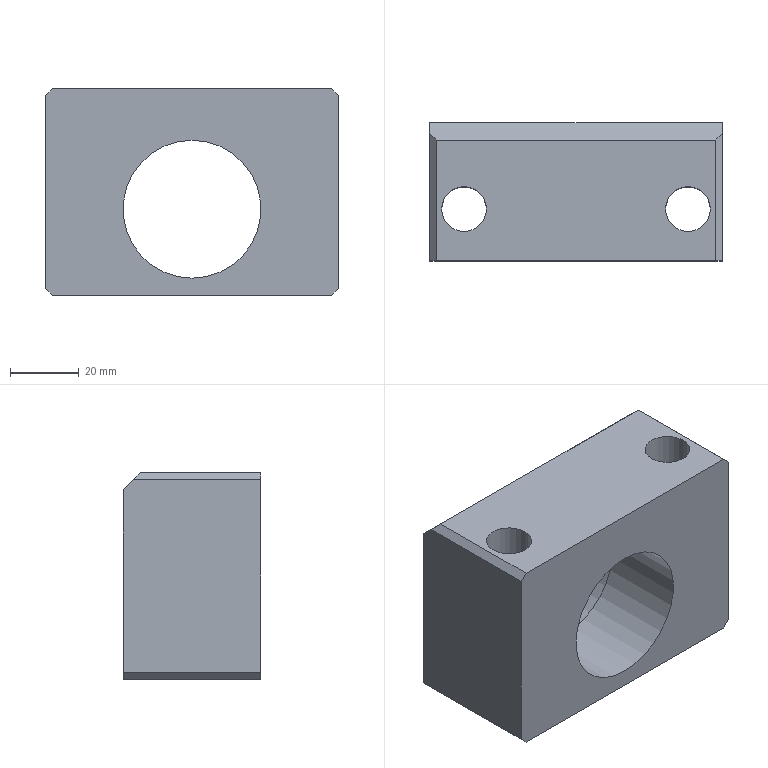Part | NX | features solid 2 | 1 solid | 16 faces | box 85 x 40 x 60 mm | volume 131435 mm3 | plane 12 | cylinder 4 | commonest cylinder face diameters 13 x2 40 x1 45 x1
STEP:
#1=CARTESIAN_POINT('',(521.,750.,75.));
#2=VERTEX_POINT('',#1);
#3=CARTESIAN_POINT('',(527.5,750.,75.));
#4=DIRECTION('',(0.,0.,-1.));
#5=DIRECTION('',(-1.,0.,0.));
#6=AXIS2_PLACEMENT_3D('',#3,#4,#5);
#7=CIRCLE('',#6,6.5);
#8=EDGE_CURVE('',#2,#2,#7,.T.);
#9=ORIENTED_EDGE('',*,*,#8,.F.);
#10=EDGE_LOOP('',(#9));
#11=FACE_BOUND('',#10,.T.);
#12=CARTESIAN_POINT('',(456.,750.,75.));
#13=VERTEX_POINT('',#12);
#14=CARTESIAN_POINT('',(462.5,750.,75.));
#15=DIRECTION('',(0.,0.,-1.));
#16=DIRECTION('',(-1.,0.,0.));
#17=AXIS2_PLACEMENT_3D('',#14,#15,#16);
#18=CIRCLE('',#17,6.5);
#19=EDGE_CURVE('',#13,#13,#18,.T.);
#20=ORIENTED_EDGE('',*,*,#19,.F.);
#21=EDGE_LOOP('',(#20));
#22=FACE_BOUND('',#21,.T.);
#23=CARTESIAN_POINT('',(535.5,735.,75.));
#24=VERTEX_POINT('',#23);
#25=CARTESIAN_POINT('',(454.5,735.,75.));
#26=VERTEX_POINT('',#25);
#27=CARTESIAN_POINT('',(495.,735.,75.));
#28=DIRECTION('',(-1.,0.,0.));
#29=VECTOR('',#28,1000.);
#30=LINE('',#27,#29);
#31=EDGE_CURVE('',#24,#26,#30,.T.);
#32=ORIENTED_EDGE('',*,*,#31,.T.);
#33=CARTESIAN_POINT('',(454.5,775.,75.));
#34=VERTEX_POINT('',#33);
#35=CARTESIAN_POINT('',(454.5,755.,75.));
#36=DIRECTION('',(0.,-1.,0.));
#37=VECTOR('',#36,1000.);
#38=LINE('',#35,#37);
#39=EDGE_CURVE('',#34,#26,#38,.T.);
#40=ORIENTED_EDGE('',*,*,#39,.F.);
#41=CARTESIAN_POINT('',(535.5,775.,75.));
#42=VERTEX_POINT('',#41);
#43=CARTESIAN_POINT('',(495.,775.,75.));
#44=DIRECTION('',(1.,0.,0.));
#45=VECTOR('',#44,1000.);
#46=LINE('',#43,#45);
#47=EDGE_CURVE('',#34,#42,#46,.T.);
#48=ORIENTED_EDGE('',*,*,#47,.T.);
#49=CARTESIAN_POINT('',(535.5,755.,75.));
#50=DIRECTION('',(0.,1.,0.));
#51=VECTOR('',#50,1000.);
#52=LINE('',#49,#51);
#53=EDGE_CURVE('',#24,#42,#52,.T.);
#54=ORIENTED_EDGE('',*,*,#53,.F.);
#55=EDGE_LOOP('',(#32,#40,#48,#54));
#56=FACE_BOUND('',#55,.T.);
#57=CARTESIAN_POINT('',(495.,755.,75.));
#58=DIRECTION('',(0.,0.,-1.));
#59=DIRECTION('',(1.,0.,0.));
#60=AXIS2_PLACEMENT_3D('',#57,#58,#59);
#61=PLANE('',#60);
#62=ADVANCED_FACE('',(#11,#22,#56),#61,.T.);
#63=CARTESIAN_POINT('',(495.,735.,120.));
#64=VERTEX_POINT('',#63);
#65=CARTESIAN_POINT('',(495.,735.,100.));
#66=DIRECTION('',(0.,1.,0.));
#67=DIRECTION('',(0.,0.,1.));
#68=AXIS2_PLACEMENT_3D('',#65,#66,#67);
#69=CIRCLE('',#68,20.);
#70=EDGE_CURVE('',#64,#64,#69,.T.);
#71=ORIENTED_EDGE('',*,*,#70,.T.);
#72=EDGE_LOOP('',(#71));
#73=FACE_BOUND('',#72,.T.);
#74=CARTESIAN_POINT('',(452.5,735.,133.));
#75=VERTEX_POINT('',#74);
#76=CARTESIAN_POINT('',(452.5,735.,77.));
#77=VERTEX_POINT('',#76);
#78=CARTESIAN_POINT('',(452.5,735.,135.));
#79=DIRECTION('',(0.,0.,-1.));
#80=VECTOR('',#79,1000.);
#81=LINE('',#78,#80);
#82=EDGE_CURVE('',#75,#77,#81,.T.);
#83=ORIENTED_EDGE('',*,*,#82,.T.);
#84=CARTESIAN_POINT('',(444.75,735.,84.75));
#85=DIRECTION('',(0.7071,0.,-0.7071));
#86=VECTOR('',#85,1000.);
#87=LINE('',#84,#86);
#88=EDGE_CURVE('',#26,#77,#87,.F.);
#89=ORIENTED_EDGE('',*,*,#88,.F.);
#90=ORIENTED_EDGE('',*,*,#31,.F.);
#91=CARTESIAN_POINT('',(537.5,735.,77.));
#92=VERTEX_POINT('',#91);
#93=CARTESIAN_POINT('',(545.25,735.,84.75));
#94=DIRECTION('',(0.7071,0.,0.7071));
#95=VECTOR('',#94,1000.);
#96=LINE('',#93,#95);
#97=EDGE_CURVE('',#92,#24,#96,.F.);
#98=ORIENTED_EDGE('',*,*,#97,.F.);
#99=CARTESIAN_POINT('',(537.5,735.,133.));
#100=VERTEX_POINT('',#99);
#101=CARTESIAN_POINT('',(537.5,735.,135.));
#102=DIRECTION('',(0.,0.,-1.));
#103=VECTOR('',#102,1000.);
#104=LINE('',#101,#103);
#105=EDGE_CURVE('',#100,#92,#104,.T.);
#106=ORIENTED_EDGE('',*,*,#105,.F.);
#107=CARTESIAN_POINT('',(535.5,735.,135.));
#108=VERTEX_POINT('',#107);
#109=CARTESIAN_POINT('',(515.25,735.,155.25));
#110=DIRECTION('',(-0.7071,0.,0.7071));
#111=VECTOR('',#110,1000.);
#112=LINE('',#109,#111);
#113=EDGE_CURVE('',#108,#100,#112,.F.);
#114=ORIENTED_EDGE('',*,*,#113,.F.);
#115=CARTESIAN_POINT('',(454.5,735.,135.));
#116=VERTEX_POINT('',#115);
#117=CARTESIAN_POINT('',(495.,735.,135.));
#118=DIRECTION('',(1.,0.,0.));
#119=VECTOR('',#118,1000.);
#120=LINE('',#117,#119);
#121=EDGE_CURVE('',#116,#108,#120,.T.);
#122=ORIENTED_EDGE('',*,*,#121,.F.);
#123=CARTESIAN_POINT('',(474.75,735.,155.25));
#124=DIRECTION('',(-0.7071,0.,-0.7071));
#125=VECTOR('',#124,1000.);
#126=LINE('',#123,#125);
#127=EDGE_CURVE('',#75,#116,#126,.F.);
#128=ORIENTED_EDGE('',*,*,#127,.F.);
#129=EDGE_LOOP('',(#83,#89,#90,#98,#106,#114,#122,#128));
#130=FACE_BOUND('',#129,.T.);
#131=CARTESIAN_POINT('',(495.,735.,135.));
#132=DIRECTION('',(0.,-1.,0.));
#133=DIRECTION('',(0.,0.,1.));
#134=AXIS2_PLACEMENT_3D('',#131,#132,#133);
#135=PLANE('',#134);
#136=ADVANCED_FACE('',(#73,#130),#135,.T.);
#137=CARTESIAN_POINT('',(452.5,775.,130.));
#138=VERTEX_POINT('',#137);
#139=CARTESIAN_POINT('',(452.5,772.,133.));
#140=VERTEX_POINT('',#139);
#141=CARTESIAN_POINT('',(452.5,762.5,142.5));
#142=DIRECTION('',(0.,0.7071,-0.7071));
#143=VECTOR('',#142,1000.);
#144=LINE('',#141,#143);
#145=EDGE_CURVE('',#138,#140,#144,.F.);
#146=ORIENTED_EDGE('',*,*,#145,.F.);
#147=CARTESIAN_POINT('',(452.5,775.,77.));
#148=VERTEX_POINT('',#147);
#149=CARTESIAN_POINT('',(452.5,775.,135.));
#150=DIRECTION('',(0.,0.,-1.));
#151=VECTOR('',#150,1000.);
#152=LINE('',#149,#151);
#153=EDGE_CURVE('',#138,#148,#152,.T.);
#154=ORIENTED_EDGE('',*,*,#153,.T.);
#155=CARTESIAN_POINT('',(452.5,755.,77.));
#156=DIRECTION('',(0.,1.,0.));
#157=VECTOR('',#156,1000.);
#158=LINE('',#155,#157);
#159=EDGE_CURVE('',#77,#148,#158,.T.);
#160=ORIENTED_EDGE('',*,*,#159,.F.);
#161=ORIENTED_EDGE('',*,*,#82,.F.);
#162=CARTESIAN_POINT('',(452.5,755.,133.));
#163=DIRECTION('',(0.,-1.,0.));
#164=VECTOR('',#163,1000.);
#165=LINE('',#162,#164);
#166=EDGE_CURVE('',#140,#75,#165,.T.);
#167=ORIENTED_EDGE('',*,*,#166,.F.);
#168=EDGE_LOOP('',(#146,#154,#160,#161,#167));
#169=FACE_BOUND('',#168,.T.);
#170=CARTESIAN_POINT('',(452.5,755.,135.));
#171=DIRECTION('',(-1.,0.,0.));
#172=DIRECTION('',(0.,0.,-1.));
#173=AXIS2_PLACEMENT_3D('',#170,#171,#172);
#174=PLANE('',#173);
#175=ADVANCED_FACE('',(#169),#174,.T.);
#176=CARTESIAN_POINT('',(495.,775.,122.5));
#177=VERTEX_POINT('',#176);
#178=CARTESIAN_POINT('',(495.,775.,100.));
#179=DIRECTION('',(0.,1.,0.));
#180=DIRECTION('',(0.,0.,1.));
#181=AXIS2_PLACEMENT_3D('',#178,#179,#180);
#182=CIRCLE('',#181,22.5);
#183=EDGE_CURVE('',#177,#177,#182,.T.);
#184=ORIENTED_EDGE('',*,*,#183,.F.);
#185=EDGE_LOOP('',(#184));
#186=FACE_BOUND('',#185,.T.);
#187=ORIENTED_EDGE('',*,*,#47,.F.);
#188=CARTESIAN_POINT('',(444.75,775.,84.75));
#189=DIRECTION('',(-0.7071,0.,0.7071));
#190=VECTOR('',#189,1000.);
#191=LINE('',#188,#190);
#192=EDGE_CURVE('',#148,#34,#191,.F.);
#193=ORIENTED_EDGE('',*,*,#192,.F.);
#194=ORIENTED_EDGE('',*,*,#153,.F.);
#195=CARTESIAN_POINT('',(537.5,775.,130.));
#196=VERTEX_POINT('',#195);
#197=CARTESIAN_POINT('',(495.,775.,130.));
#198=DIRECTION('',(-1.,0.,0.));
#199=VECTOR('',#198,1000.);
#200=LINE('',#197,#199);
#201=EDGE_CURVE('',#196,#138,#200,.T.);
#202=ORIENTED_EDGE('',*,*,#201,.F.);
#203=CARTESIAN_POINT('',(537.5,775.,77.));
#204=VERTEX_POINT('',#203);
#205=CARTESIAN_POINT('',(537.5,775.,135.));
#206=DIRECTION('',(0.,0.,-1.));
#207=VECTOR('',#206,1000.);
#208=LINE('',#205,#207);
#209=EDGE_CURVE('',#196,#204,#208,.T.);
#210=ORIENTED_EDGE('',*,*,#209,.T.);
#211=CARTESIAN_POINT('',(545.25,775.,84.75));
#212=DIRECTION('',(-0.7071,0.,-0.7071));
#213=VECTOR('',#212,1000.);
#214=LINE('',#211,#213);
#215=EDGE_CURVE('',#42,#204,#214,.F.);
#216=ORIENTED_EDGE('',*,*,#215,.F.);
#217=EDGE_LOOP('',(#187,#193,#194,#202,#210,#216));
#218=FACE_BOUND('',#217,.T.);
#219=CARTESIAN_POINT('',(495.,775.,135.));
#220=DIRECTION('',(0.,1.,0.));
#221=DIRECTION('',(0.,0.,-1.));
#222=AXIS2_PLACEMENT_3D('',#219,#220,#221);
#223=PLANE('',#222);
#224=ADVANCED_FACE('',(#186,#218),#223,.T.);
#225=CARTESIAN_POINT('',(521.,750.,135.));
#226=VERTEX_POINT('',#225);
#227=CARTESIAN_POINT('',(527.5,750.,135.));
#228=DIRECTION('',(0.,0.,-1.));
#229=DIRECTION('',(-1.,0.,0.));
#230=AXIS2_PLACEMENT_3D('',#227,#228,#229);
#231=CIRCLE('',#230,6.5);
#232=EDGE_CURVE('',#226,#226,#231,.T.);
#233=ORIENTED_EDGE('',*,*,#232,.T.);
#234=EDGE_LOOP('',(#233));
#235=FACE_BOUND('',#234,.T.);
#236=CARTESIAN_POINT('',(456.,750.,135.));
#237=VERTEX_POINT('',#236);
#238=CARTESIAN_POINT('',(462.5,750.,135.));
#239=DIRECTION('',(0.,0.,-1.));
#240=DIRECTION('',(-1.,0.,0.));
#241=AXIS2_PLACEMENT_3D('',#238,#239,#240);
#242=CIRCLE('',#241,6.5);
#243=EDGE_CURVE('',#237,#237,#242,.T.);
#244=ORIENTED_EDGE('',*,*,#243,.T.);
#245=EDGE_LOOP('',(#244));
#246=FACE_BOUND('',#245,.T.);
#247=ORIENTED_EDGE('',*,*,#121,.T.);
#248=CARTESIAN_POINT('',(535.5,770.,135.));
#249=VERTEX_POINT('',#248);
#250=CARTESIAN_POINT('',(535.5,755.,135.));
#251=DIRECTION('',(0.,-1.,0.));
#252=VECTOR('',#251,1000.);
#253=LINE('',#250,#252);
#254=EDGE_CURVE('',#249,#108,#253,.T.);
#255=ORIENTED_EDGE('',*,*,#254,.F.);
#256=CARTESIAN_POINT('',(454.5,770.,135.));
#257=VERTEX_POINT('',#256);
#258=CARTESIAN_POINT('',(495.,770.,135.));
#259=DIRECTION('',(1.,0.,0.));
#260=VECTOR('',#259,1000.);
#261=LINE('',#258,#260);
#262=EDGE_CURVE('',#257,#249,#261,.T.);
#263=ORIENTED_EDGE('',*,*,#262,.F.);
#264=CARTESIAN_POINT('',(454.5,755.,135.));
#265=DIRECTION('',(0.,1.,0.));
#266=VECTOR('',#265,1000.);
#267=LINE('',#264,#266);
#268=EDGE_CURVE('',#116,#257,#267,.T.);
#269=ORIENTED_EDGE('',*,*,#268,.F.);
#270=EDGE_LOOP('',(#247,#255,#263,#269));
#271=FACE_BOUND('',#270,.T.);
#272=CARTESIAN_POINT('',(495.,755.,135.));
#273=DIRECTION('',(0.,0.,1.));
#274=DIRECTION('',(-1.,0.,0.));
#275=AXIS2_PLACEMENT_3D('',#272,#273,#274);
#276=PLANE('',#275);
#277=ADVANCED_FACE('',(#235,#246,#271),#276,.T.);
#278=ORIENTED_EDGE('',*,*,#105,.T.);
#279=CARTESIAN_POINT('',(537.5,755.,77.));
#280=DIRECTION('',(0.,-1.,0.));
#281=VECTOR('',#280,1000.);
#282=LINE('',#279,#281);
#283=EDGE_CURVE('',#204,#92,#282,.T.);
#284=ORIENTED_EDGE('',*,*,#283,.F.);
#285=ORIENTED_EDGE('',*,*,#209,.F.);
#286=CARTESIAN_POINT('',(537.5,772.,133.));
#287=VERTEX_POINT('',#286);
#288=CARTESIAN_POINT('',(537.5,762.5,142.5));
#289=DIRECTION('',(0.,-0.7071,0.7071));
#290=VECTOR('',#289,1000.);
#291=LINE('',#288,#290);
#292=EDGE_CURVE('',#287,#196,#291,.F.);
#293=ORIENTED_EDGE('',*,*,#292,.F.);
#294=CARTESIAN_POINT('',(537.5,755.,133.));
#295=DIRECTION('',(0.,1.,0.));
#296=VECTOR('',#295,1000.);
#297=LINE('',#294,#296);
#298=EDGE_CURVE('',#100,#287,#297,.T.);
#299=ORIENTED_EDGE('',*,*,#298,.F.);
#300=EDGE_LOOP('',(#278,#284,#285,#293,#299));
#301=FACE_BOUND('',#300,.T.);
#302=CARTESIAN_POINT('',(537.5,755.,135.));
#303=DIRECTION('',(1.,0.,0.));
#304=DIRECTION('',(0.,0.,1.));
#305=AXIS2_PLACEMENT_3D('',#302,#303,#304);
#306=PLANE('',#305);
#307=ADVANCED_FACE('',(#301),#306,.T.);
#308=ORIENTED_EDGE('',*,*,#262,.T.);
#309=CARTESIAN_POINT('',(525.333,759.833,145.167));
#310=DIRECTION('',(-0.5774,-0.5774,0.5774));
#311=VECTOR('',#310,1000.);
#312=LINE('',#309,#311);
#313=EDGE_CURVE('',#287,#249,#312,.T.);
#314=ORIENTED_EDGE('',*,*,#313,.F.);
#315=ORIENTED_EDGE('',*,*,#292,.T.);
#316=ORIENTED_EDGE('',*,*,#201,.T.);
#317=ORIENTED_EDGE('',*,*,#145,.T.);
#318=CARTESIAN_POINT('',(464.667,759.833,145.167));
#319=DIRECTION('',(-0.5774,0.5774,-0.5774));
#320=VECTOR('',#319,1000.);
#321=LINE('',#318,#320);
#322=EDGE_CURVE('',#257,#140,#321,.T.);
#323=ORIENTED_EDGE('',*,*,#322,.F.);
#324=EDGE_LOOP('',(#308,#314,#315,#316,#317,#323));
#325=FACE_BOUND('',#324,.T.);
#326=CARTESIAN_POINT('',(495.,775.,130.));
#327=DIRECTION('',(0.,-0.7071,-0.7071));
#328=DIRECTION('',(0.,-0.7071,0.7071));
#329=AXIS2_PLACEMENT_3D('',#326,#327,#328);
#330=PLANE('',#329);
#331=ADVANCED_FACE('',(#325),#330,.F.);
#332=ORIENTED_EDGE('',*,*,#70,.F.);
#333=EDGE_LOOP('',(#332));
#334=FACE_BOUND('',#333,.T.);
#335=CARTESIAN_POINT('',(495.,760.,120.));
#336=VERTEX_POINT('',#335);
#337=CARTESIAN_POINT('',(495.,760.,100.));
#338=DIRECTION('',(0.,1.,0.));
#339=DIRECTION('',(0.,0.,1.));
#340=AXIS2_PLACEMENT_3D('',#337,#338,#339);
#341=CIRCLE('',#340,20.);
#342=EDGE_CURVE('',#336,#336,#341,.T.);
#343=ORIENTED_EDGE('',*,*,#342,.T.);
#344=EDGE_LOOP('',(#343));
#345=FACE_BOUND('',#344,.T.);
#346=CARTESIAN_POINT('',(495.,735.,100.));
#347=DIRECTION('',(0.,-1.,0.));
#348=DIRECTION('',(0.,0.,1.));
#349=AXIS2_PLACEMENT_3D('',#346,#347,#348);
#350=CYLINDRICAL_SURFACE('',#349,20.);
#351=ADVANCED_FACE('',(#334,#345),#350,.F.);
#352=ORIENTED_EDGE('',*,*,#342,.F.);
#353=EDGE_LOOP('',(#352));
#354=FACE_BOUND('',#353,.T.);
#355=CARTESIAN_POINT('',(495.,760.,122.5));
#356=VERTEX_POINT('',#355);
#357=CARTESIAN_POINT('',(495.,760.,100.));
#358=DIRECTION('',(0.,1.,0.));
#359=DIRECTION('',(0.,0.,1.));
#360=AXIS2_PLACEMENT_3D('',#357,#358,#359);
#361=CIRCLE('',#360,22.5);
#362=EDGE_CURVE('',#356,#356,#361,.T.);
#363=ORIENTED_EDGE('',*,*,#362,.T.);
#364=EDGE_LOOP('',(#363));
#365=FACE_BOUND('',#364,.T.);
#366=CARTESIAN_POINT('',(495.,760.,100.));
#367=DIRECTION('',(0.,-1.,0.));
#368=DIRECTION('',(0.,0.,1.));
#369=AXIS2_PLACEMENT_3D('',#366,#367,#368);
#370=PLANE('',#369);
#371=ADVANCED_FACE('',(#354,#365),#370,.F.);
#372=ORIENTED_EDGE('',*,*,#362,.F.);
#373=EDGE_LOOP('',(#372));
#374=FACE_BOUND('',#373,.T.);
#375=ORIENTED_EDGE('',*,*,#183,.T.);
#376=EDGE_LOOP('',(#375));
#377=FACE_BOUND('',#376,.T.);
#378=CARTESIAN_POINT('',(495.,775.,100.));
#379=DIRECTION('',(0.,-1.,0.));
#380=DIRECTION('',(0.,0.,1.));
#381=AXIS2_PLACEMENT_3D('',#378,#379,#380);
#382=CYLINDRICAL_SURFACE('',#381,22.5);
#383=ADVANCED_FACE('',(#374,#377),#382,.F.);
#384=ORIENTED_EDGE('',*,*,#88,.T.);
#385=ORIENTED_EDGE('',*,*,#159,.T.);
#386=ORIENTED_EDGE('',*,*,#192,.T.);
#387=ORIENTED_EDGE('',*,*,#39,.T.);
#388=EDGE_LOOP('',(#384,#385,#386,#387));
#389=FACE_BOUND('',#388,.T.);
#390=CARTESIAN_POINT('',(452.5,755.,77.));
#391=DIRECTION('',(0.7071,0.,0.7071));
#392=DIRECTION('',(-0.7071,0.,0.7071));
#393=AXIS2_PLACEMENT_3D('',#390,#391,#392);
#394=PLANE('',#393);
#395=ADVANCED_FACE('',(#389),#394,.F.);
#396=ORIENTED_EDGE('',*,*,#215,.T.);
#397=ORIENTED_EDGE('',*,*,#283,.T.);
#398=ORIENTED_EDGE('',*,*,#97,.T.);
#399=ORIENTED_EDGE('',*,*,#53,.T.);
#400=EDGE_LOOP('',(#396,#397,#398,#399));
#401=FACE_BOUND('',#400,.T.);
#402=CARTESIAN_POINT('',(537.5,755.,77.));
#403=DIRECTION('',(-0.7071,0.,0.7071));
#404=DIRECTION('',(-0.7071,0.,-0.7071));
#405=AXIS2_PLACEMENT_3D('',#402,#403,#404);
#406=PLANE('',#405);
#407=ADVANCED_FACE('',(#401),#406,.F.);
#408=ORIENTED_EDGE('',*,*,#113,.T.);
#409=ORIENTED_EDGE('',*,*,#298,.T.);
#410=ORIENTED_EDGE('',*,*,#313,.T.);
#411=ORIENTED_EDGE('',*,*,#254,.T.);
#412=EDGE_LOOP('',(#408,#409,#410,#411));
#413=FACE_BOUND('',#412,.T.);
#414=CARTESIAN_POINT('',(537.5,755.,133.));
#415=DIRECTION('',(-0.7071,0.,-0.7071));
#416=DIRECTION('',(0.7071,0.,-0.7071));
#417=AXIS2_PLACEMENT_3D('',#414,#415,#416);
#418=PLANE('',#417);
#419=ADVANCED_FACE('',(#413),#418,.F.);
#420=ORIENTED_EDGE('',*,*,#322,.T.);
#421=ORIENTED_EDGE('',*,*,#166,.T.);
#422=ORIENTED_EDGE('',*,*,#127,.T.);
#423=ORIENTED_EDGE('',*,*,#268,.T.);
#424=EDGE_LOOP('',(#420,#421,#422,#423));
#425=FACE_BOUND('',#424,.T.);
#426=CARTESIAN_POINT('',(452.5,755.,133.));
#427=DIRECTION('',(0.7071,0.,-0.7071));
#428=DIRECTION('',(0.7071,0.,0.7071));
#429=AXIS2_PLACEMENT_3D('',#426,#427,#428);
#430=PLANE('',#429);
#431=ADVANCED_FACE('',(#425),#430,.F.);
#432=ORIENTED_EDGE('',*,*,#243,.F.);
#433=EDGE_LOOP('',(#432));
#434=FACE_BOUND('',#433,.T.);
#435=ORIENTED_EDGE('',*,*,#19,.T.);
#436=EDGE_LOOP('',(#435));
#437=FACE_BOUND('',#436,.T.);
#438=CARTESIAN_POINT('',(462.5,750.,75.));
#439=DIRECTION('',(0.,0.,1.));
#440=DIRECTION('',(-1.,0.,0.));
#441=AXIS2_PLACEMENT_3D('',#438,#439,#440);
#442=CYLINDRICAL_SURFACE('',#441,6.5);
#443=ADVANCED_FACE('',(#434,#437),#442,.F.);
#444=ORIENTED_EDGE('',*,*,#232,.F.);
#445=EDGE_LOOP('',(#444));
#446=FACE_BOUND('',#445,.T.);
#447=ORIENTED_EDGE('',*,*,#8,.T.);
#448=EDGE_LOOP('',(#447));
#449=FACE_BOUND('',#448,.T.);
#450=CARTESIAN_POINT('',(527.5,750.,75.));
#451=DIRECTION('',(0.,0.,1.));
#452=DIRECTION('',(-1.,0.,0.));
#453=AXIS2_PLACEMENT_3D('',#450,#451,#452);
#454=CYLINDRICAL_SURFACE('',#453,6.5);
#455=ADVANCED_FACE('',(#446,#449),#454,.F.);
#456=CLOSED_SHELL('',(#62,#136,#175,#224,#277,#307,#331,#351,#371,#383,#395,#407,#419,#431,#443,#455));
#457=MANIFOLD_SOLID_BREP('',#456);
#458=(LENGTH_UNIT()NAMED_UNIT(*)SI_UNIT(.MILLI.,.METRE.));
#459=UNCERTAINTY_MEASURE_WITH_UNIT(LENGTH_MEASURE(0.00001),#458,'','');
#460=(NAMED_UNIT(*)PLANE_ANGLE_UNIT()SI_UNIT($,.RADIAN.));
#461=(NAMED_UNIT(*)SI_UNIT($,.STERADIAN.)SOLID_ANGLE_UNIT());
#462=(GEOMETRIC_REPRESENTATION_CONTEXT(3)GLOBAL_UNCERTAINTY_ASSIGNED_CONTEXT((#459))GLOBAL_UNIT_ASSIGNED_CONTEXT((#458,#460,#461))REPRESENTATION_CONTEXT('',''));
#463=ADVANCED_BREP_SHAPE_REPRESENTATION('',(#457),#462);